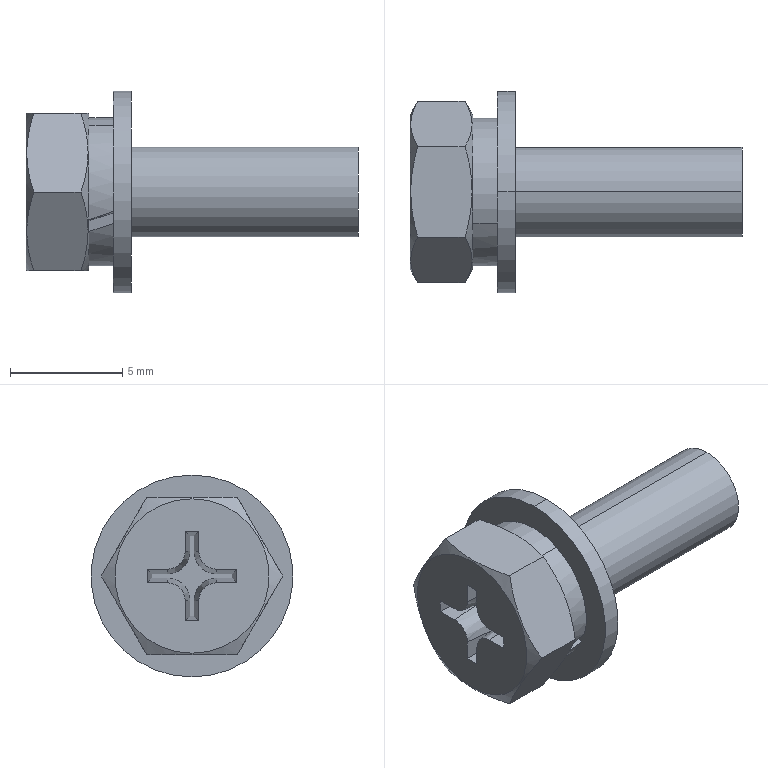Part | SolidWorks | features BaseBody 3 | 3 solids | 54 faces | box 14.8 x 9 x 9 mm | volume 319.757 mm3 | plane 28 | cylinder 14 | cone 10 | torus 2 | commonest cylinder face diameters 4.4 x3 6.6 x3 3.8 x2 4 x2 4.3 x2 9 x2